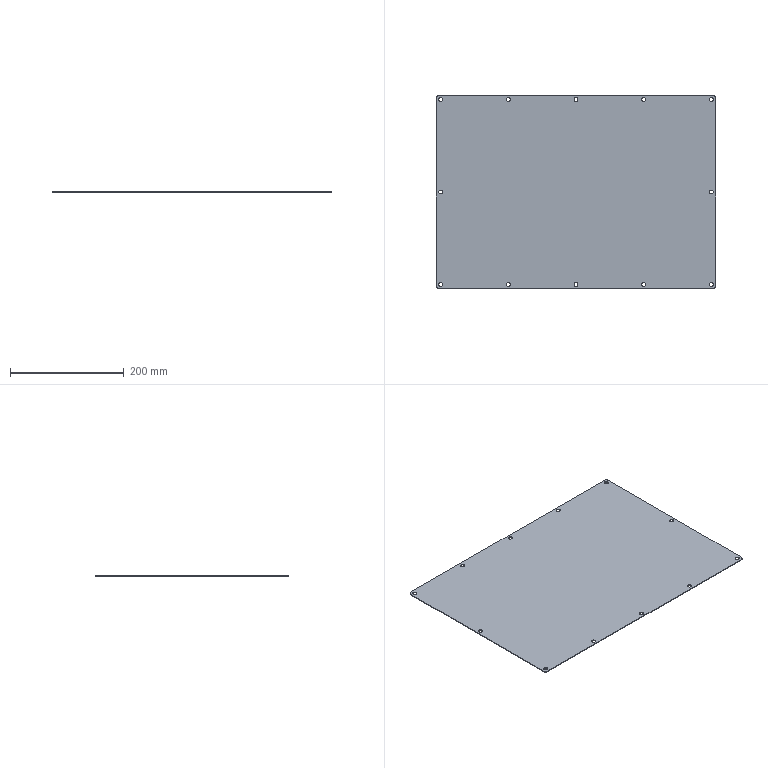Part | SolidWorks | features FlatPattern 1, SMBaseFlange 1, SheetMetal 1 | 1 solid | 34 faces | box 490 x 340 x 1.2 mm | volume 199340 mm3 | cylinder 28 | plane 6 | commonest cylinder face diameters 7 x24 10 x4
STEP:
#1=CARTESIAN_POINT('',(235.2,162.5,1.2));
#2=VERTEX_POINT('',#1);
#3=CARTESIAN_POINT('',(242.2,162.5,1.2));
#4=VERTEX_POINT('',#3);
#5=CARTESIAN_POINT('',(238.7,162.5,1.2));
#6=DIRECTION('',(0.,0.,1.));
#7=DIRECTION('',(1.,0.,0.));
#8=AXIS2_PLACEMENT_3D('',#5,#6,#7);
#9=CIRCLE('',#8,3.5);
#10=EDGE_CURVE('',#2,#4,#9,.T.);
#11=ORIENTED_EDGE('',*,*,#10,.T.);
#12=CARTESIAN_POINT('',(242.2,162.5,0.));
#13=VERTEX_POINT('',#12);
#14=CARTESIAN_POINT('',(242.2,162.5,1.2));
#15=DIRECTION('',(0.,0.,-1.));
#16=VECTOR('',#15,1000.);
#17=LINE('',#14,#16);
#18=EDGE_CURVE('',#4,#13,#17,.T.);
#19=ORIENTED_EDGE('',*,*,#18,.T.);
#20=CARTESIAN_POINT('',(235.2,162.5,0.));
#21=VERTEX_POINT('',#20);
#22=CARTESIAN_POINT('',(238.7,162.5,0.));
#23=DIRECTION('',(0.,0.,1.));
#24=DIRECTION('',(1.,0.,0.));
#25=AXIS2_PLACEMENT_3D('',#22,#23,#24);
#26=CIRCLE('',#25,3.5);
#27=EDGE_CURVE('',#21,#13,#26,.T.);
#28=ORIENTED_EDGE('',*,*,#27,.F.);
#29=CARTESIAN_POINT('',(235.2,162.5,1.2));
#30=DIRECTION('',(0.,0.,-1.));
#31=VECTOR('',#30,1000.);
#32=LINE('',#29,#31);
#33=EDGE_CURVE('',#2,#21,#32,.T.);
#34=ORIENTED_EDGE('',*,*,#33,.F.);
#35=EDGE_LOOP('',(#11,#19,#28,#34));
#36=FACE_OUTER_BOUND('',#35,.T.);
#37=CARTESIAN_POINT('',(238.7,162.5,1.2));
#38=DIRECTION('',(0.,0.,-1.));
#39=DIRECTION('',(-1.,0.,0.));
#40=AXIS2_PLACEMENT_3D('',#37,#38,#39);
#41=CYLINDRICAL_SURFACE('',#40,3.5);
#42=ADVANCED_FACE('',(#36),#41,.F.);
#43=CARTESIAN_POINT('',(235.2,-162.5,1.2));
#44=VERTEX_POINT('',#43);
#45=CARTESIAN_POINT('',(242.2,-162.5,1.2));
#46=VERTEX_POINT('',#45);
#47=CARTESIAN_POINT('',(238.7,-162.5,1.2));
#48=DIRECTION('',(0.,0.,1.));
#49=DIRECTION('',(1.,0.,0.));
#50=AXIS2_PLACEMENT_3D('',#47,#48,#49);
#51=CIRCLE('',#50,3.5);
#52=EDGE_CURVE('',#44,#46,#51,.T.);
#53=ORIENTED_EDGE('',*,*,#52,.T.);
#54=CARTESIAN_POINT('',(242.2,-162.5,0.));
#55=VERTEX_POINT('',#54);
#56=CARTESIAN_POINT('',(242.2,-162.5,1.2));
#57=DIRECTION('',(0.,0.,-1.));
#58=VECTOR('',#57,1000.);
#59=LINE('',#56,#58);
#60=EDGE_CURVE('',#46,#55,#59,.T.);
#61=ORIENTED_EDGE('',*,*,#60,.T.);
#62=CARTESIAN_POINT('',(235.2,-162.5,0.));
#63=VERTEX_POINT('',#62);
#64=CARTESIAN_POINT('',(238.7,-162.5,0.));
#65=DIRECTION('',(0.,0.,1.));
#66=DIRECTION('',(1.,0.,0.));
#67=AXIS2_PLACEMENT_3D('',#64,#65,#66);
#68=CIRCLE('',#67,3.5);
#69=EDGE_CURVE('',#63,#55,#68,.T.);
#70=ORIENTED_EDGE('',*,*,#69,.F.);
#71=CARTESIAN_POINT('',(235.2,-162.5,1.2));
#72=DIRECTION('',(0.,0.,-1.));
#73=VECTOR('',#72,1000.);
#74=LINE('',#71,#73);
#75=EDGE_CURVE('',#44,#63,#74,.T.);
#76=ORIENTED_EDGE('',*,*,#75,.F.);
#77=EDGE_LOOP('',(#53,#61,#70,#76));
#78=FACE_OUTER_BOUND('',#77,.T.);
#79=CARTESIAN_POINT('',(238.7,-162.5,1.2));
#80=DIRECTION('',(0.,0.,-1.));
#81=DIRECTION('',(-1.,0.,0.));
#82=AXIS2_PLACEMENT_3D('',#79,#80,#81);
#83=CYLINDRICAL_SURFACE('',#82,3.5);
#84=ADVANCED_FACE('',(#78),#83,.F.);
#85=CARTESIAN_POINT('',(116.45,162.5,1.2));
#86=VERTEX_POINT('',#85);
#87=CARTESIAN_POINT('',(123.45,162.5,1.2));
#88=VERTEX_POINT('',#87);
#89=CARTESIAN_POINT('',(119.95,162.5,1.2));
#90=DIRECTION('',(0.,0.,1.));
#91=DIRECTION('',(1.,0.,0.));
#92=AXIS2_PLACEMENT_3D('',#89,#90,#91);
#93=CIRCLE('',#92,3.5);
#94=EDGE_CURVE('',#86,#88,#93,.T.);
#95=ORIENTED_EDGE('',*,*,#94,.T.);
#96=CARTESIAN_POINT('',(123.45,162.5,0.));
#97=VERTEX_POINT('',#96);
#98=CARTESIAN_POINT('',(123.45,162.5,1.2));
#99=DIRECTION('',(0.,0.,-1.));
#100=VECTOR('',#99,1000.);
#101=LINE('',#98,#100);
#102=EDGE_CURVE('',#88,#97,#101,.T.);
#103=ORIENTED_EDGE('',*,*,#102,.T.);
#104=CARTESIAN_POINT('',(116.45,162.5,0.));
#105=VERTEX_POINT('',#104);
#106=CARTESIAN_POINT('',(119.95,162.5,0.));
#107=DIRECTION('',(0.,0.,1.));
#108=DIRECTION('',(1.,0.,0.));
#109=AXIS2_PLACEMENT_3D('',#106,#107,#108);
#110=CIRCLE('',#109,3.5);
#111=EDGE_CURVE('',#105,#97,#110,.T.);
#112=ORIENTED_EDGE('',*,*,#111,.F.);
#113=CARTESIAN_POINT('',(116.45,162.5,1.2));
#114=DIRECTION('',(0.,0.,-1.));
#115=VECTOR('',#114,1000.);
#116=LINE('',#113,#115);
#117=EDGE_CURVE('',#86,#105,#116,.T.);
#118=ORIENTED_EDGE('',*,*,#117,.F.);
#119=EDGE_LOOP('',(#95,#103,#112,#118));
#120=FACE_OUTER_BOUND('',#119,.T.);
#121=CARTESIAN_POINT('',(119.95,162.5,1.2));
#122=DIRECTION('',(0.,0.,-1.));
#123=DIRECTION('',(-1.,0.,0.));
#124=AXIS2_PLACEMENT_3D('',#121,#122,#123);
#125=CYLINDRICAL_SURFACE('',#124,3.5);
#126=ADVANCED_FACE('',(#120),#125,.F.);
#127=CARTESIAN_POINT('',(116.45,-162.5,1.2));
#128=VERTEX_POINT('',#127);
#129=CARTESIAN_POINT('',(123.45,-162.5,1.2));
#130=VERTEX_POINT('',#129);
#131=CARTESIAN_POINT('',(119.95,-162.5,1.2));
#132=DIRECTION('',(0.,0.,1.));
#133=DIRECTION('',(1.,0.,0.));
#134=AXIS2_PLACEMENT_3D('',#131,#132,#133);
#135=CIRCLE('',#134,3.5);
#136=EDGE_CURVE('',#128,#130,#135,.T.);
#137=ORIENTED_EDGE('',*,*,#136,.T.);
#138=CARTESIAN_POINT('',(123.45,-162.5,0.));
#139=VERTEX_POINT('',#138);
#140=CARTESIAN_POINT('',(123.45,-162.5,1.2));
#141=DIRECTION('',(0.,0.,-1.));
#142=VECTOR('',#141,1000.);
#143=LINE('',#140,#142);
#144=EDGE_CURVE('',#130,#139,#143,.T.);
#145=ORIENTED_EDGE('',*,*,#144,.T.);
#146=CARTESIAN_POINT('',(116.45,-162.5,0.));
#147=VERTEX_POINT('',#146);
#148=CARTESIAN_POINT('',(119.95,-162.5,0.));
#149=DIRECTION('',(0.,0.,1.));
#150=DIRECTION('',(1.,0.,0.));
#151=AXIS2_PLACEMENT_3D('',#148,#149,#150);
#152=CIRCLE('',#151,3.5);
#153=EDGE_CURVE('',#147,#139,#152,.T.);
#154=ORIENTED_EDGE('',*,*,#153,.F.);
#155=CARTESIAN_POINT('',(116.45,-162.5,1.2));
#156=DIRECTION('',(0.,0.,-1.));
#157=VECTOR('',#156,1000.);
#158=LINE('',#155,#157);
#159=EDGE_CURVE('',#128,#147,#158,.T.);
#160=ORIENTED_EDGE('',*,*,#159,.F.);
#161=EDGE_LOOP('',(#137,#145,#154,#160));
#162=FACE_OUTER_BOUND('',#161,.T.);
#163=CARTESIAN_POINT('',(119.95,-162.5,1.2));
#164=DIRECTION('',(0.,0.,-1.));
#165=DIRECTION('',(-1.,0.,0.));
#166=AXIS2_PLACEMENT_3D('',#163,#164,#165);
#167=CYLINDRICAL_SURFACE('',#166,3.5);
#168=ADVANCED_FACE('',(#162),#167,.F.);
#169=CARTESIAN_POINT('',(-2.3,162.5,1.2));
#170=VERTEX_POINT('',#169);
#171=CARTESIAN_POINT('',(4.7,162.5,1.2));
#172=VERTEX_POINT('',#171);
#173=CARTESIAN_POINT('',(1.2,162.5,1.2));
#174=DIRECTION('',(0.,0.,1.));
#175=DIRECTION('',(1.,0.,0.));
#176=AXIS2_PLACEMENT_3D('',#173,#174,#175);
#177=CIRCLE('',#176,3.5);
#178=EDGE_CURVE('',#170,#172,#177,.T.);
#179=ORIENTED_EDGE('',*,*,#178,.T.);
#180=CARTESIAN_POINT('',(4.7,162.5,0.));
#181=VERTEX_POINT('',#180);
#182=CARTESIAN_POINT('',(4.7,162.5,1.2));
#183=DIRECTION('',(0.,0.,-1.));
#184=VECTOR('',#183,1000.);
#185=LINE('',#182,#184);
#186=EDGE_CURVE('',#172,#181,#185,.T.);
#187=ORIENTED_EDGE('',*,*,#186,.T.);
#188=CARTESIAN_POINT('',(-2.3,162.5,0.));
#189=VERTEX_POINT('',#188);
#190=CARTESIAN_POINT('',(1.2,162.5,0.));
#191=DIRECTION('',(0.,0.,1.));
#192=DIRECTION('',(1.,0.,0.));
#193=AXIS2_PLACEMENT_3D('',#190,#191,#192);
#194=CIRCLE('',#193,3.5);
#195=EDGE_CURVE('',#189,#181,#194,.T.);
#196=ORIENTED_EDGE('',*,*,#195,.F.);
#197=CARTESIAN_POINT('',(-2.3,162.5,1.2));
#198=DIRECTION('',(0.,0.,-1.));
#199=VECTOR('',#198,1000.);
#200=LINE('',#197,#199);
#201=EDGE_CURVE('',#170,#189,#200,.T.);
#202=ORIENTED_EDGE('',*,*,#201,.F.);
#203=EDGE_LOOP('',(#179,#187,#196,#202));
#204=FACE_OUTER_BOUND('',#203,.T.);
#205=CARTESIAN_POINT('',(1.2,162.5,1.2));
#206=DIRECTION('',(0.,0.,-1.));
#207=DIRECTION('',(-1.,0.,0.));
#208=AXIS2_PLACEMENT_3D('',#205,#206,#207);
#209=CYLINDRICAL_SURFACE('',#208,3.5);
#210=ADVANCED_FACE('',(#204),#209,.F.);
#211=CARTESIAN_POINT('',(-2.3,-162.5,1.2));
#212=VERTEX_POINT('',#211);
#213=CARTESIAN_POINT('',(4.7,-162.5,1.2));
#214=VERTEX_POINT('',#213);
#215=CARTESIAN_POINT('',(1.2,-162.5,1.2));
#216=DIRECTION('',(0.,0.,1.));
#217=DIRECTION('',(1.,0.,0.));
#218=AXIS2_PLACEMENT_3D('',#215,#216,#217);
#219=CIRCLE('',#218,3.5);
#220=EDGE_CURVE('',#212,#214,#219,.T.);
#221=ORIENTED_EDGE('',*,*,#220,.T.);
#222=CARTESIAN_POINT('',(4.7,-162.5,0.));
#223=VERTEX_POINT('',#222);
#224=CARTESIAN_POINT('',(4.7,-162.5,1.2));
#225=DIRECTION('',(0.,0.,-1.));
#226=VECTOR('',#225,1000.);
#227=LINE('',#224,#226);
#228=EDGE_CURVE('',#214,#223,#227,.T.);
#229=ORIENTED_EDGE('',*,*,#228,.T.);
#230=CARTESIAN_POINT('',(-2.3,-162.5,0.));
#231=VERTEX_POINT('',#230);
#232=CARTESIAN_POINT('',(1.2,-162.5,0.));
#233=DIRECTION('',(0.,0.,1.));
#234=DIRECTION('',(1.,0.,0.));
#235=AXIS2_PLACEMENT_3D('',#232,#233,#234);
#236=CIRCLE('',#235,3.5);
#237=EDGE_CURVE('',#231,#223,#236,.T.);
#238=ORIENTED_EDGE('',*,*,#237,.F.);
#239=CARTESIAN_POINT('',(-2.3,-162.5,1.2));
#240=DIRECTION('',(0.,0.,-1.));
#241=VECTOR('',#240,1000.);
#242=LINE('',#239,#241);
#243=EDGE_CURVE('',#212,#231,#242,.T.);
#244=ORIENTED_EDGE('',*,*,#243,.F.);
#245=EDGE_LOOP('',(#221,#229,#238,#244));
#246=FACE_OUTER_BOUND('',#245,.T.);
#247=CARTESIAN_POINT('',(1.2,-162.5,1.2));
#248=DIRECTION('',(0.,0.,-1.));
#249=DIRECTION('',(-1.,0.,0.));
#250=AXIS2_PLACEMENT_3D('',#247,#248,#249);
#251=CYLINDRICAL_SURFACE('',#250,3.5);
#252=ADVANCED_FACE('',(#246),#251,.F.);
#253=CARTESIAN_POINT('',(-121.05,162.5,1.2));
#254=VERTEX_POINT('',#253);
#255=CARTESIAN_POINT('',(-114.05,162.5,1.2));
#256=VERTEX_POINT('',#255);
#257=CARTESIAN_POINT('',(-117.55,162.5,1.2));
#258=DIRECTION('',(0.,0.,1.));
#259=DIRECTION('',(1.,0.,0.));
#260=AXIS2_PLACEMENT_3D('',#257,#258,#259);
#261=CIRCLE('',#260,3.5);
#262=EDGE_CURVE('',#254,#256,#261,.T.);
#263=ORIENTED_EDGE('',*,*,#262,.T.);
#264=CARTESIAN_POINT('',(-114.05,162.5,0.));
#265=VERTEX_POINT('',#264);
#266=CARTESIAN_POINT('',(-114.05,162.5,1.2));
#267=DIRECTION('',(0.,0.,-1.));
#268=VECTOR('',#267,1000.);
#269=LINE('',#266,#268);
#270=EDGE_CURVE('',#256,#265,#269,.T.);
#271=ORIENTED_EDGE('',*,*,#270,.T.);
#272=CARTESIAN_POINT('',(-121.05,162.5,0.));
#273=VERTEX_POINT('',#272);
#274=CARTESIAN_POINT('',(-117.55,162.5,0.));
#275=DIRECTION('',(0.,0.,1.));
#276=DIRECTION('',(1.,0.,0.));
#277=AXIS2_PLACEMENT_3D('',#274,#275,#276);
#278=CIRCLE('',#277,3.5);
#279=EDGE_CURVE('',#273,#265,#278,.T.);
#280=ORIENTED_EDGE('',*,*,#279,.F.);
#281=CARTESIAN_POINT('',(-121.05,162.5,1.2));
#282=DIRECTION('',(0.,0.,-1.));
#283=VECTOR('',#282,1000.);
#284=LINE('',#281,#283);
#285=EDGE_CURVE('',#254,#273,#284,.T.);
#286=ORIENTED_EDGE('',*,*,#285,.F.);
#287=EDGE_LOOP('',(#263,#271,#280,#286));
#288=FACE_OUTER_BOUND('',#287,.T.);
#289=CARTESIAN_POINT('',(-117.55,162.5,1.2));
#290=DIRECTION('',(0.,0.,-1.));
#291=DIRECTION('',(-1.,0.,0.));
#292=AXIS2_PLACEMENT_3D('',#289,#290,#291);
#293=CYLINDRICAL_SURFACE('',#292,3.5);
#294=ADVANCED_FACE('',(#288),#293,.F.);
#295=CARTESIAN_POINT('',(-121.05,-162.5,1.2));
#296=VERTEX_POINT('',#295);
#297=CARTESIAN_POINT('',(-114.05,-162.5,1.2));
#298=VERTEX_POINT('',#297);
#299=CARTESIAN_POINT('',(-117.55,-162.5,1.2));
#300=DIRECTION('',(0.,0.,1.));
#301=DIRECTION('',(1.,0.,0.));
#302=AXIS2_PLACEMENT_3D('',#299,#300,#301);
#303=CIRCLE('',#302,3.5);
#304=EDGE_CURVE('',#296,#298,#303,.T.);
#305=ORIENTED_EDGE('',*,*,#304,.T.);
#306=CARTESIAN_POINT('',(-114.05,-162.5,0.));
#307=VERTEX_POINT('',#306);
#308=CARTESIAN_POINT('',(-114.05,-162.5,1.2));
#309=DIRECTION('',(0.,0.,-1.));
#310=VECTOR('',#309,1000.);
#311=LINE('',#308,#310);
#312=EDGE_CURVE('',#298,#307,#311,.T.);
#313=ORIENTED_EDGE('',*,*,#312,.T.);
#314=CARTESIAN_POINT('',(-121.05,-162.5,0.));
#315=VERTEX_POINT('',#314);
#316=CARTESIAN_POINT('',(-117.55,-162.5,0.));
#317=DIRECTION('',(0.,0.,1.));
#318=DIRECTION('',(1.,0.,0.));
#319=AXIS2_PLACEMENT_3D('',#316,#317,#318);
#320=CIRCLE('',#319,3.5);
#321=EDGE_CURVE('',#315,#307,#320,.T.);
#322=ORIENTED_EDGE('',*,*,#321,.F.);
#323=CARTESIAN_POINT('',(-121.05,-162.5,1.2));
#324=DIRECTION('',(0.,0.,-1.));
#325=VECTOR('',#324,1000.);
#326=LINE('',#323,#325);
#327=EDGE_CURVE('',#296,#315,#326,.T.);
#328=ORIENTED_EDGE('',*,*,#327,.F.);
#329=EDGE_LOOP('',(#305,#313,#322,#328));
#330=FACE_OUTER_BOUND('',#329,.T.);
#331=CARTESIAN_POINT('',(-117.55,-162.5,1.2));
#332=DIRECTION('',(0.,0.,-1.));
#333=DIRECTION('',(-1.,0.,0.));
#334=AXIS2_PLACEMENT_3D('',#331,#332,#333);
#335=CYLINDRICAL_SURFACE('',#334,3.5);
#336=ADVANCED_FACE('',(#330),#335,.F.);
#337=CARTESIAN_POINT('',(235.2,0.,1.2));
#338=VERTEX_POINT('',#337);
#339=CARTESIAN_POINT('',(242.2,0.,1.2));
#340=VERTEX_POINT('',#339);
#341=CARTESIAN_POINT('',(238.7,0.,1.2));
#342=DIRECTION('',(0.,0.,1.));
#343=DIRECTION('',(1.,0.,0.));
#344=AXIS2_PLACEMENT_3D('',#341,#342,#343);
#345=CIRCLE('',#344,3.5);
#346=EDGE_CURVE('',#338,#340,#345,.T.);
#347=ORIENTED_EDGE('',*,*,#346,.T.);
#348=CARTESIAN_POINT('',(242.2,0.,0.));
#349=VERTEX_POINT('',#348);
#350=CARTESIAN_POINT('',(242.2,0.,1.2));
#351=DIRECTION('',(0.,0.,-1.));
#352=VECTOR('',#351,1000.);
#353=LINE('',#350,#352);
#354=EDGE_CURVE('',#340,#349,#353,.T.);
#355=ORIENTED_EDGE('',*,*,#354,.T.);
#356=CARTESIAN_POINT('',(235.2,0.,0.));
#357=VERTEX_POINT('',#356);
#358=CARTESIAN_POINT('',(238.7,0.,0.));
#359=DIRECTION('',(0.,0.,1.));
#360=DIRECTION('',(1.,0.,0.));
#361=AXIS2_PLACEMENT_3D('',#358,#359,#360);
#362=CIRCLE('',#361,3.5);
#363=EDGE_CURVE('',#357,#349,#362,.T.);
#364=ORIENTED_EDGE('',*,*,#363,.F.);
#365=CARTESIAN_POINT('',(235.2,0.,1.2));
#366=DIRECTION('',(0.,0.,-1.));
#367=VECTOR('',#366,1000.);
#368=LINE('',#365,#367);
#369=EDGE_CURVE('',#338,#357,#368,.T.);
#370=ORIENTED_EDGE('',*,*,#369,.F.);
#371=EDGE_LOOP('',(#347,#355,#364,#370));
#372=FACE_OUTER_BOUND('',#371,.T.);
#373=CARTESIAN_POINT('',(238.7,0.,1.2));
#374=DIRECTION('',(0.,0.,-1.));
#375=DIRECTION('',(-1.,0.,0.));
#376=AXIS2_PLACEMENT_3D('',#373,#374,#375);
#377=CYLINDRICAL_SURFACE('',#376,3.5);
#378=ADVANCED_FACE('',(#372),#377,.F.);
#379=CARTESIAN_POINT('',(-239.8,162.5,1.2));
#380=VERTEX_POINT('',#379);
#381=CARTESIAN_POINT('',(-232.8,162.5,1.2));
#382=VERTEX_POINT('',#381);
#383=CARTESIAN_POINT('',(-236.3,162.5,1.2));
#384=DIRECTION('',(0.,0.,1.));
#385=DIRECTION('',(1.,0.,0.));
#386=AXIS2_PLACEMENT_3D('',#383,#384,#385);
#387=CIRCLE('',#386,3.5);
#388=EDGE_CURVE('',#380,#382,#387,.T.);
#389=ORIENTED_EDGE('',*,*,#388,.T.);
#390=CARTESIAN_POINT('',(-232.8,162.5,0.));
#391=VERTEX_POINT('',#390);
#392=CARTESIAN_POINT('',(-232.8,162.5,1.2));
#393=DIRECTION('',(0.,0.,-1.));
#394=VECTOR('',#393,1000.);
#395=LINE('',#392,#394);
#396=EDGE_CURVE('',#382,#391,#395,.T.);
#397=ORIENTED_EDGE('',*,*,#396,.T.);
#398=CARTESIAN_POINT('',(-239.8,162.5,0.));
#399=VERTEX_POINT('',#398);
#400=CARTESIAN_POINT('',(-236.3,162.5,0.));
#401=DIRECTION('',(0.,0.,1.));
#402=DIRECTION('',(1.,0.,0.));
#403=AXIS2_PLACEMENT_3D('',#400,#401,#402);
#404=CIRCLE('',#403,3.5);
#405=EDGE_CURVE('',#399,#391,#404,.T.);
#406=ORIENTED_EDGE('',*,*,#405,.F.);
#407=CARTESIAN_POINT('',(-239.8,162.5,1.2));
#408=DIRECTION('',(0.,0.,-1.));
#409=VECTOR('',#408,1000.);
#410=LINE('',#407,#409);
#411=EDGE_CURVE('',#380,#399,#410,.T.);
#412=ORIENTED_EDGE('',*,*,#411,.F.);
#413=EDGE_LOOP('',(#389,#397,#406,#412));
#414=FACE_OUTER_BOUND('',#413,.T.);
#415=CARTESIAN_POINT('',(-236.3,162.5,1.2));
#416=DIRECTION('',(0.,0.,-1.));
#417=DIRECTION('',(-1.,0.,0.));
#418=AXIS2_PLACEMENT_3D('',#415,#416,#417);
#419=CYLINDRICAL_SURFACE('',#418,3.5);
#420=ADVANCED_FACE('',(#414),#419,.F.);
#421=CARTESIAN_POINT('',(-239.8,0.,1.2));
#422=VERTEX_POINT('',#421);
#423=CARTESIAN_POINT('',(-232.8,0.,1.2));
#424=VERTEX_POINT('',#423);
#425=CARTESIAN_POINT('',(-236.3,0.,1.2));
#426=DIRECTION('',(0.,0.,1.));
#427=DIRECTION('',(1.,0.,0.));
#428=AXIS2_PLACEMENT_3D('',#425,#426,#427);
#429=CIRCLE('',#428,3.5);
#430=EDGE_CURVE('',#422,#424,#429,.T.);
#431=ORIENTED_EDGE('',*,*,#430,.T.);
#432=CARTESIAN_POINT('',(-232.8,0.,0.));
#433=VERTEX_POINT('',#432);
#434=CARTESIAN_POINT('',(-232.8,0.,1.2));
#435=DIRECTION('',(0.,0.,-1.));
#436=VECTOR('',#435,1000.);
#437=LINE('',#434,#436);
#438=EDGE_CURVE('',#424,#433,#437,.T.);
#439=ORIENTED_EDGE('',*,*,#438,.T.);
#440=CARTESIAN_POINT('',(-239.8,0.,0.));
#441=VERTEX_POINT('',#440);
#442=CARTESIAN_POINT('',(-236.3,0.,0.));
#443=DIRECTION('',(0.,0.,1.));
#444=DIRECTION('',(1.,0.,0.));
#445=AXIS2_PLACEMENT_3D('',#442,#443,#444);
#446=CIRCLE('',#445,3.5);
#447=EDGE_CURVE('',#441,#433,#446,.T.);
#448=ORIENTED_EDGE('',*,*,#447,.F.);
#449=CARTESIAN_POINT('',(-239.8,0.,1.2));
#450=DIRECTION('',(0.,0.,-1.));
#451=VECTOR('',#450,1000.);
#452=LINE('',#449,#451);
#453=EDGE_CURVE('',#422,#441,#452,.T.);
#454=ORIENTED_EDGE('',*,*,#453,.F.);
#455=EDGE_LOOP('',(#431,#439,#448,#454));
#456=FACE_OUTER_BOUND('',#455,.T.);
#457=CARTESIAN_POINT('',(-236.3,0.,1.2));
#458=DIRECTION('',(0.,0.,-1.));
#459=DIRECTION('',(-1.,0.,0.));
#460=AXIS2_PLACEMENT_3D('',#457,#458,#459);
#461=CYLINDRICAL_SURFACE('',#460,3.5);
#462=ADVANCED_FACE('',(#456),#461,.F.);
#463=CARTESIAN_POINT('',(-239.8,-162.5,1.2));
#464=VERTEX_POINT('',#463);
#465=CARTESIAN_POINT('',(-232.8,-162.5,1.2));
#466=VERTEX_POINT('',#465);
#467=CARTESIAN_POINT('',(-236.3,-162.5,1.2));
#468=DIRECTION('',(0.,0.,1.));
#469=DIRECTION('',(1.,0.,0.));
#470=AXIS2_PLACEMENT_3D('',#467,#468,#469);
#471=CIRCLE('',#470,3.5);
#472=EDGE_CURVE('',#464,#466,#471,.T.);
#473=ORIENTED_EDGE('',*,*,#472,.T.);
#474=CARTESIAN_POINT('',(-232.8,-162.5,0.));
#475=VERTEX_POINT('',#474);
#476=CARTESIAN_POINT('',(-232.8,-162.5,1.2));
#477=DIRECTION('',(0.,0.,-1.));
#478=VECTOR('',#477,1000.);
#479=LINE('',#476,#478);
#480=EDGE_CURVE('',#466,#475,#479,.T.);
#481=ORIENTED_EDGE('',*,*,#480,.T.);
#482=CARTESIAN_POINT('',(-239.8,-162.5,0.));
#483=VERTEX_POINT('',#482);
#484=CARTESIAN_POINT('',(-236.3,-162.5,0.));
#485=DIRECTION('',(0.,0.,1.));
#486=DIRECTION('',(1.,0.,0.));
#487=AXIS2_PLACEMENT_3D('',#484,#485,#486);
#488=CIRCLE('',#487,3.5);
#489=EDGE_CURVE('',#483,#475,#488,.T.);
#490=ORIENTED_EDGE('',*,*,#489,.F.);
#491=CARTESIAN_POINT('',(-239.8,-162.5,1.2));
#492=DIRECTION('',(0.,0.,-1.));
#493=VECTOR('',#492,1000.);
#494=LINE('',#491,#493);
#495=EDGE_CURVE('',#464,#483,#494,.T.);
#496=ORIENTED_EDGE('',*,*,#495,.F.);
#497=EDGE_LOOP('',(#473,#481,#490,#496));
#498=FACE_OUTER_BOUND('',#497,.T.);
#499=CARTESIAN_POINT('',(-236.3,-162.5,1.2));
#500=DIRECTION('',(0.,0.,-1.));
#501=DIRECTION('',(-1.,0.,0.));
#502=AXIS2_PLACEMENT_3D('',#499,#500,#501);
#503=CYLINDRICAL_SURFACE('',#502,3.5);
#504=ADVANCED_FACE('',(#498),#503,.F.);
#505=ORIENTED_EDGE('',*,*,#52,.F.);
#506=CARTESIAN_POINT('',(238.7,-162.5,1.2));
#507=DIRECTION('',(0.,0.,1.));
#508=DIRECTION('',(1.,0.,0.));
#509=AXIS2_PLACEMENT_3D('',#506,#507,#508);
#510=CIRCLE('',#509,3.5);
#511=EDGE_CURVE('',#46,#44,#510,.T.);
#512=ORIENTED_EDGE('',*,*,#511,.F.);
#513=EDGE_LOOP('',(#505,#512));
#514=FACE_BOUND('',#513,.T.);
#515=ORIENTED_EDGE('',*,*,#136,.F.);
#516=CARTESIAN_POINT('',(119.95,-162.5,1.2));
#517=DIRECTION('',(0.,0.,1.));
#518=DIRECTION('',(1.,0.,0.));
#519=AXIS2_PLACEMENT_3D('',#516,#517,#518);
#520=CIRCLE('',#519,3.5);
#521=EDGE_CURVE('',#130,#128,#520,.T.);
#522=ORIENTED_EDGE('',*,*,#521,.F.);
#523=EDGE_LOOP('',(#515,#522));
#524=FACE_BOUND('',#523,.T.);
#525=ORIENTED_EDGE('',*,*,#220,.F.);
#526=CARTESIAN_POINT('',(1.2,-162.5,1.2));
#527=DIRECTION('',(0.,0.,1.));
#528=DIRECTION('',(1.,0.,0.));
#529=AXIS2_PLACEMENT_3D('',#526,#527,#528);
#530=CIRCLE('',#529,3.5);
#531=EDGE_CURVE('',#214,#212,#530,.T.);
#532=ORIENTED_EDGE('',*,*,#531,.F.);
#533=EDGE_LOOP('',(#525,#532));
#534=FACE_BOUND('',#533,.T.);
#535=ORIENTED_EDGE('',*,*,#304,.F.);
#536=CARTESIAN_POINT('',(-117.55,-162.5,1.2));
#537=DIRECTION('',(0.,0.,1.));
#538=DIRECTION('',(1.,0.,0.));
#539=AXIS2_PLACEMENT_3D('',#536,#537,#538);
#540=CIRCLE('',#539,3.5);
#541=EDGE_CURVE('',#298,#296,#540,.T.);
#542=ORIENTED_EDGE('',*,*,#541,.F.);
#543=EDGE_LOOP('',(#535,#542));
#544=FACE_BOUND('',#543,.T.);
#545=ORIENTED_EDGE('',*,*,#388,.F.);
#546=CARTESIAN_POINT('',(-236.3,162.5,1.2));
#547=DIRECTION('',(0.,0.,1.));
#548=DIRECTION('',(1.,0.,0.));
#549=AXIS2_PLACEMENT_3D('',#546,#547,#548);
#550=CIRCLE('',#549,3.5);
#551=EDGE_CURVE('',#382,#380,#550,.T.);
#552=ORIENTED_EDGE('',*,*,#551,.F.);
#553=EDGE_LOOP('',(#545,#552));
#554=FACE_BOUND('',#553,.T.);
#555=ORIENTED_EDGE('',*,*,#472,.F.);
#556=CARTESIAN_POINT('',(-236.3,-162.5,1.2));
#557=DIRECTION('',(0.,0.,1.));
#558=DIRECTION('',(1.,0.,0.));
#559=AXIS2_PLACEMENT_3D('',#556,#557,#558);
#560=CIRCLE('',#559,3.5);
#561=EDGE_CURVE('',#466,#464,#560,.T.);
#562=ORIENTED_EDGE('',*,*,#561,.F.);
#563=EDGE_LOOP('',(#555,#562));
#564=FACE_BOUND('',#563,.T.);
#565=CARTESIAN_POINT('',(241.2,-170.,1.2));
#566=VERTEX_POINT('',#565);
#567=CARTESIAN_POINT('',(246.2,-165.,1.2));
#568=VERTEX_POINT('',#567);
#569=CARTESIAN_POINT('',(241.2,-165.,1.2));
#570=DIRECTION('',(0.,0.,1.));
#571=DIRECTION('',(1.,0.,0.));
#572=AXIS2_PLACEMENT_3D('',#569,#570,#571);
#573=CIRCLE('',#572,5.);
#574=EDGE_CURVE('',#566,#568,#573,.T.);
#575=ORIENTED_EDGE('',*,*,#574,.T.);
#576=CARTESIAN_POINT('',(246.2,165.,1.2));
#577=VERTEX_POINT('',#576);
#578=CARTESIAN_POINT('',(246.2,-165.,1.2));
#579=DIRECTION('',(0.,1.,0.));
#580=VECTOR('',#579,1000.);
#581=LINE('',#578,#580);
#582=EDGE_CURVE('',#568,#577,#581,.T.);
#583=ORIENTED_EDGE('',*,*,#582,.T.);
#584=CARTESIAN_POINT('',(241.2,170.,1.2));
#585=VERTEX_POINT('',#584);
#586=CARTESIAN_POINT('',(241.2,165.,1.2));
#587=DIRECTION('',(0.,0.,1.));
#588=DIRECTION('',(-1.,0.,0.));
#589=AXIS2_PLACEMENT_3D('',#586,#587,#588);
#590=CIRCLE('',#589,5.);
#591=EDGE_CURVE('',#577,#585,#590,.T.);
#592=ORIENTED_EDGE('',*,*,#591,.T.);
#593=CARTESIAN_POINT('',(-238.8,170.,1.2));
#594=VERTEX_POINT('',#593);
#595=CARTESIAN_POINT('',(-238.8,170.,1.2));
#596=DIRECTION('',(-1.,0.,0.));
#597=VECTOR('',#596,1000.);
#598=LINE('',#595,#597);
#599=EDGE_CURVE('',#585,#594,#598,.T.);
#600=ORIENTED_EDGE('',*,*,#599,.T.);
#601=CARTESIAN_POINT('',(-243.8,165.,1.2));
#602=VERTEX_POINT('',#601);
#603=CARTESIAN_POINT('',(-238.8,165.,1.2));
#604=DIRECTION('',(0.,0.,1.));
#605=DIRECTION('',(-1.,0.,0.));
#606=AXIS2_PLACEMENT_3D('',#603,#604,#605);
#607=CIRCLE('',#606,5.);
#608=EDGE_CURVE('',#594,#602,#607,.T.);
#609=ORIENTED_EDGE('',*,*,#608,.T.);
#610=CARTESIAN_POINT('',(-243.8,-165.,1.2));
#611=VERTEX_POINT('',#610);
#612=CARTESIAN_POINT('',(-243.8,-165.,1.2));
#613=DIRECTION('',(0.,-1.,0.));
#614=VECTOR('',#613,1000.);
#615=LINE('',#612,#614);
#616=EDGE_CURVE('',#602,#611,#615,.T.);
#617=ORIENTED_EDGE('',*,*,#616,.T.);
#618=CARTESIAN_POINT('',(-238.8,-170.,1.2));
#619=VERTEX_POINT('',#618);
#620=CARTESIAN_POINT('',(-238.8,-165.,1.2));
#621=DIRECTION('',(0.,0.,1.));
#622=DIRECTION('',(-1.,0.,0.));
#623=AXIS2_PLACEMENT_3D('',#620,#621,#622);
#624=CIRCLE('',#623,5.);
#625=EDGE_CURVE('',#611,#619,#624,.T.);
#626=ORIENTED_EDGE('',*,*,#625,.T.);
#627=CARTESIAN_POINT('',(-238.8,-170.,1.2));
#628=DIRECTION('',(1.,0.,0.));
#629=VECTOR('',#628,1000.);
#630=LINE('',#627,#629);
#631=EDGE_CURVE('',#619,#566,#630,.T.);
#632=ORIENTED_EDGE('',*,*,#631,.T.);
#633=EDGE_LOOP('',(#575,#583,#592,#600,#609,#617,#626,#632));
#634=FACE_OUTER_BOUND('',#633,.T.);
#635=ORIENTED_EDGE('',*,*,#430,.F.);
#636=CARTESIAN_POINT('',(-236.3,0.,1.2));
#637=DIRECTION('',(0.,0.,1.));
#638=DIRECTION('',(1.,0.,0.));
#639=AXIS2_PLACEMENT_3D('',#636,#637,#638);
#640=CIRCLE('',#639,3.5);
#641=EDGE_CURVE('',#424,#422,#640,.T.);
#642=ORIENTED_EDGE('',*,*,#641,.F.);
#643=EDGE_LOOP('',(#635,#642));
#644=FACE_BOUND('',#643,.T.);
#645=ORIENTED_EDGE('',*,*,#346,.F.);
#646=CARTESIAN_POINT('',(238.7,0.,1.2));
#647=DIRECTION('',(0.,0.,1.));
#648=DIRECTION('',(1.,0.,0.));
#649=AXIS2_PLACEMENT_3D('',#646,#647,#648);
#650=CIRCLE('',#649,3.5);
#651=EDGE_CURVE('',#340,#338,#650,.T.);
#652=ORIENTED_EDGE('',*,*,#651,.F.);
#653=EDGE_LOOP('',(#645,#652));
#654=FACE_BOUND('',#653,.T.);
#655=ORIENTED_EDGE('',*,*,#262,.F.);
#656=CARTESIAN_POINT('',(-117.55,162.5,1.2));
#657=DIRECTION('',(0.,0.,1.));
#658=DIRECTION('',(1.,0.,0.));
#659=AXIS2_PLACEMENT_3D('',#656,#657,#658);
#660=CIRCLE('',#659,3.5);
#661=EDGE_CURVE('',#256,#254,#660,.T.);
#662=ORIENTED_EDGE('',*,*,#661,.F.);
#663=EDGE_LOOP('',(#655,#662));
#664=FACE_BOUND('',#663,.T.);
#665=ORIENTED_EDGE('',*,*,#178,.F.);
#666=CARTESIAN_POINT('',(1.2,162.5,1.2));
#667=DIRECTION('',(0.,0.,1.));
#668=DIRECTION('',(1.,0.,0.));
#669=AXIS2_PLACEMENT_3D('',#666,#667,#668);
#670=CIRCLE('',#669,3.5);
#671=EDGE_CURVE('',#172,#170,#670,.T.);
#672=ORIENTED_EDGE('',*,*,#671,.F.);
#673=EDGE_LOOP('',(#665,#672));
#674=FACE_BOUND('',#673,.T.);
#675=ORIENTED_EDGE('',*,*,#94,.F.);
#676=CARTESIAN_POINT('',(119.95,162.5,1.2));
#677=DIRECTION('',(0.,0.,1.));
#678=DIRECTION('',(1.,0.,0.));
#679=AXIS2_PLACEMENT_3D('',#676,#677,#678);
#680=CIRCLE('',#679,3.5);
#681=EDGE_CURVE('',#88,#86,#680,.T.);
#682=ORIENTED_EDGE('',*,*,#681,.F.);
#683=EDGE_LOOP('',(#675,#682));
#684=FACE_BOUND('',#683,.T.);
#685=ORIENTED_EDGE('',*,*,#10,.F.);
#686=CARTESIAN_POINT('',(238.7,162.5,1.2));
#687=DIRECTION('',(0.,0.,1.));
#688=DIRECTION('',(1.,0.,0.));
#689=AXIS2_PLACEMENT_3D('',#686,#687,#688);
#690=CIRCLE('',#689,3.5);
#691=EDGE_CURVE('',#4,#2,#690,.T.);
#692=ORIENTED_EDGE('',*,*,#691,.F.);
#693=EDGE_LOOP('',(#685,#692));
#694=FACE_BOUND('',#693,.T.);
#695=CARTESIAN_POINT('',(241.2,-165.,1.2));
#696=DIRECTION('',(0.,0.,1.));
#697=DIRECTION('',(1.,0.,0.));
#698=AXIS2_PLACEMENT_3D('',#695,#696,#697);
#699=PLANE('',#698);
#700=ADVANCED_FACE('',(#514,#524,#534,#544,#554,#564,#634,#644,#654,#664,#674,#684,#694),#699,.T.);
#701=CARTESIAN_POINT('',(241.2,-170.,0.));
#702=VERTEX_POINT('',#701);
#703=CARTESIAN_POINT('',(246.2,-165.,0.));
#704=VERTEX_POINT('',#703);
#705=CARTESIAN_POINT('',(241.2,-165.,0.));
#706=DIRECTION('',(0.,0.,1.));
#707=DIRECTION('',(1.,0.,0.));
#708=AXIS2_PLACEMENT_3D('',#705,#706,#707);
#709=CIRCLE('',#708,5.);
#710=EDGE_CURVE('',#702,#704,#709,.T.);
#711=ORIENTED_EDGE('',*,*,#710,.F.);
#712=CARTESIAN_POINT('',(-238.8,-170.,0.));
#713=VERTEX_POINT('',#712);
#714=CARTESIAN_POINT('',(-238.8,-170.,0.));
#715=DIRECTION('',(1.,0.,0.));
#716=VECTOR('',#715,1000.);
#717=LINE('',#714,#716);
#718=EDGE_CURVE('',#713,#702,#717,.T.);
#719=ORIENTED_EDGE('',*,*,#718,.F.);
#720=CARTESIAN_POINT('',(-243.8,-165.,0.));
#721=VERTEX_POINT('',#720);
#722=CARTESIAN_POINT('',(-238.8,-165.,0.));
#723=DIRECTION('',(0.,0.,1.));
#724=DIRECTION('',(-1.,0.,0.));
#725=AXIS2_PLACEMENT_3D('',#722,#723,#724);
#726=CIRCLE('',#725,5.);
#727=EDGE_CURVE('',#721,#713,#726,.T.);
#728=ORIENTED_EDGE('',*,*,#727,.F.);
#729=CARTESIAN_POINT('',(-243.8,165.,0.));
#730=VERTEX_POINT('',#729);
#731=CARTESIAN_POINT('',(-243.8,-165.,0.));
#732=DIRECTION('',(0.,-1.,0.));
#733=VECTOR('',#732,1000.);
#734=LINE('',#731,#733);
#735=EDGE_CURVE('',#730,#721,#734,.T.);
#736=ORIENTED_EDGE('',*,*,#735,.F.);
#737=CARTESIAN_POINT('',(-238.8,170.,0.));
#738=VERTEX_POINT('',#737);
#739=CARTESIAN_POINT('',(-238.8,165.,0.));
#740=DIRECTION('',(0.,0.,1.));
#741=DIRECTION('',(-1.,0.,0.));
#742=AXIS2_PLACEMENT_3D('',#739,#740,#741);
#743=CIRCLE('',#742,5.);
#744=EDGE_CURVE('',#738,#730,#743,.T.);
#745=ORIENTED_EDGE('',*,*,#744,.F.);
#746=CARTESIAN_POINT('',(241.2,170.,0.));
#747=VERTEX_POINT('',#746);
#748=CARTESIAN_POINT('',(-238.8,170.,0.));
#749=DIRECTION('',(-1.,0.,0.));
#750=VECTOR('',#749,1000.);
#751=LINE('',#748,#750);
#752=EDGE_CURVE('',#747,#738,#751,.T.);
#753=ORIENTED_EDGE('',*,*,#752,.F.);
#754=CARTESIAN_POINT('',(246.2,165.,0.));
#755=VERTEX_POINT('',#754);
#756=CARTESIAN_POINT('',(241.2,165.,0.));
#757=DIRECTION('',(0.,0.,1.));
#758=DIRECTION('',(-1.,0.,0.));
#759=AXIS2_PLACEMENT_3D('',#756,#757,#758);
#760=CIRCLE('',#759,5.);
#761=EDGE_CURVE('',#755,#747,#760,.T.);
#762=ORIENTED_EDGE('',*,*,#761,.F.);
#763=CARTESIAN_POINT('',(246.2,-165.,0.));
#764=DIRECTION('',(0.,1.,0.));
#765=VECTOR('',#764,1000.);
#766=LINE('',#763,#765);
#767=EDGE_CURVE('',#704,#755,#766,.T.);
#768=ORIENTED_EDGE('',*,*,#767,.F.);
#769=EDGE_LOOP('',(#711,#719,#728,#736,#745,#753,#762,#768));
#770=FACE_OUTER_BOUND('',#769,.T.);
#771=ORIENTED_EDGE('',*,*,#489,.T.);
#772=CARTESIAN_POINT('',(-236.3,-162.5,0.));
#773=DIRECTION('',(0.,0.,1.));
#774=DIRECTION('',(1.,0.,0.));
#775=AXIS2_PLACEMENT_3D('',#772,#773,#774);
#776=CIRCLE('',#775,3.5);
#777=EDGE_CURVE('',#475,#483,#776,.T.);
#778=ORIENTED_EDGE('',*,*,#777,.T.);
#779=EDGE_LOOP('',(#771,#778));
#780=FACE_BOUND('',#779,.T.);
#781=ORIENTED_EDGE('',*,*,#447,.T.);
#782=CARTESIAN_POINT('',(-236.3,0.,0.));
#783=DIRECTION('',(0.,0.,1.));
#784=DIRECTION('',(1.,0.,0.));
#785=AXIS2_PLACEMENT_3D('',#782,#783,#784);
#786=CIRCLE('',#785,3.5);
#787=EDGE_CURVE('',#433,#441,#786,.T.);
#788=ORIENTED_EDGE('',*,*,#787,.T.);
#789=EDGE_LOOP('',(#781,#788));
#790=FACE_BOUND('',#789,.T.);
#791=ORIENTED_EDGE('',*,*,#405,.T.);
#792=CARTESIAN_POINT('',(-236.3,162.5,0.));
#793=DIRECTION('',(0.,0.,1.));
#794=DIRECTION('',(1.,0.,0.));
#795=AXIS2_PLACEMENT_3D('',#792,#793,#794);
#796=CIRCLE('',#795,3.5);
#797=EDGE_CURVE('',#391,#399,#796,.T.);
#798=ORIENTED_EDGE('',*,*,#797,.T.);
#799=EDGE_LOOP('',(#791,#798));
#800=FACE_BOUND('',#799,.T.);
#801=ORIENTED_EDGE('',*,*,#363,.T.);
#802=CARTESIAN_POINT('',(238.7,0.,0.));
#803=DIRECTION('',(0.,0.,1.));
#804=DIRECTION('',(1.,0.,0.));
#805=AXIS2_PLACEMENT_3D('',#802,#803,#804);
#806=CIRCLE('',#805,3.5);
#807=EDGE_CURVE('',#349,#357,#806,.T.);
#808=ORIENTED_EDGE('',*,*,#807,.T.);
#809=EDGE_LOOP('',(#801,#808));
#810=FACE_BOUND('',#809,.T.);
#811=ORIENTED_EDGE('',*,*,#321,.T.);
#812=CARTESIAN_POINT('',(-117.55,-162.5,0.));
#813=DIRECTION('',(0.,0.,1.));
#814=DIRECTION('',(1.,0.,0.));
#815=AXIS2_PLACEMENT_3D('',#812,#813,#814);
#816=CIRCLE('',#815,3.5);
#817=EDGE_CURVE('',#307,#315,#816,.T.);
#818=ORIENTED_EDGE('',*,*,#817,.T.);
#819=EDGE_LOOP('',(#811,#818));
#820=FACE_BOUND('',#819,.T.);
#821=ORIENTED_EDGE('',*,*,#279,.T.);
#822=CARTESIAN_POINT('',(-117.55,162.5,0.));
#823=DIRECTION('',(0.,0.,1.));
#824=DIRECTION('',(1.,0.,0.));
#825=AXIS2_PLACEMENT_3D('',#822,#823,#824);
#826=CIRCLE('',#825,3.5);
#827=EDGE_CURVE('',#265,#273,#826,.T.);
#828=ORIENTED_EDGE('',*,*,#827,.T.);
#829=EDGE_LOOP('',(#821,#828));
#830=FACE_BOUND('',#829,.T.);
#831=ORIENTED_EDGE('',*,*,#237,.T.);
#832=CARTESIAN_POINT('',(1.2,-162.5,0.));
#833=DIRECTION('',(0.,0.,1.));
#834=DIRECTION('',(1.,0.,0.));
#835=AXIS2_PLACEMENT_3D('',#832,#833,#834);
#836=CIRCLE('',#835,3.5);
#837=EDGE_CURVE('',#223,#231,#836,.T.);
#838=ORIENTED_EDGE('',*,*,#837,.T.);
#839=EDGE_LOOP('',(#831,#838));
#840=FACE_BOUND('',#839,.T.);
#841=ORIENTED_EDGE('',*,*,#195,.T.);
#842=CARTESIAN_POINT('',(1.2,162.5,0.));
#843=DIRECTION('',(0.,0.,1.));
#844=DIRECTION('',(1.,0.,0.));
#845=AXIS2_PLACEMENT_3D('',#842,#843,#844);
#846=CIRCLE('',#845,3.5);
#847=EDGE_CURVE('',#181,#189,#846,.T.);
#848=ORIENTED_EDGE('',*,*,#847,.T.);
#849=EDGE_LOOP('',(#841,#848));
#850=FACE_BOUND('',#849,.T.);
#851=ORIENTED_EDGE('',*,*,#153,.T.);
#852=CARTESIAN_POINT('',(119.95,-162.5,0.));
#853=DIRECTION('',(0.,0.,1.));
#854=DIRECTION('',(1.,0.,0.));
#855=AXIS2_PLACEMENT_3D('',#852,#853,#854);
#856=CIRCLE('',#855,3.5);
#857=EDGE_CURVE('',#139,#147,#856,.T.);
#858=ORIENTED_EDGE('',*,*,#857,.T.);
#859=EDGE_LOOP('',(#851,#858));
#860=FACE_BOUND('',#859,.T.);
#861=ORIENTED_EDGE('',*,*,#111,.T.);
#862=CARTESIAN_POINT('',(119.95,162.5,0.));
#863=DIRECTION('',(0.,0.,1.));
#864=DIRECTION('',(1.,0.,0.));
#865=AXIS2_PLACEMENT_3D('',#862,#863,#864);
#866=CIRCLE('',#865,3.5);
#867=EDGE_CURVE('',#97,#105,#866,.T.);
#868=ORIENTED_EDGE('',*,*,#867,.T.);
#869=EDGE_LOOP('',(#861,#868));
#870=FACE_BOUND('',#869,.T.);
#871=ORIENTED_EDGE('',*,*,#69,.T.);
#872=CARTESIAN_POINT('',(238.7,-162.5,0.));
#873=DIRECTION('',(0.,0.,1.));
#874=DIRECTION('',(1.,0.,0.));
#875=AXIS2_PLACEMENT_3D('',#872,#873,#874);
#876=CIRCLE('',#875,3.5);
#877=EDGE_CURVE('',#55,#63,#876,.T.);
#878=ORIENTED_EDGE('',*,*,#877,.T.);
#879=EDGE_LOOP('',(#871,#878));
#880=FACE_BOUND('',#879,.T.);
#881=ORIENTED_EDGE('',*,*,#27,.T.);
#882=CARTESIAN_POINT('',(238.7,162.5,0.));
#883=DIRECTION('',(0.,0.,1.));
#884=DIRECTION('',(1.,0.,0.));
#885=AXIS2_PLACEMENT_3D('',#882,#883,#884);
#886=CIRCLE('',#885,3.5);
#887=EDGE_CURVE('',#13,#21,#886,.T.);
#888=ORIENTED_EDGE('',*,*,#887,.T.);
#889=EDGE_LOOP('',(#881,#888));
#890=FACE_BOUND('',#889,.T.);
#891=CARTESIAN_POINT('',(241.2,-165.,0.));
#892=DIRECTION('',(0.,0.,1.));
#893=DIRECTION('',(1.,0.,0.));
#894=AXIS2_PLACEMENT_3D('',#891,#892,#893);
#895=PLANE('',#894);
#896=ADVANCED_FACE('',(#770,#780,#790,#800,#810,#820,#830,#840,#850,#860,#870,#880,#890),#895,.F.);
#897=ORIENTED_EDGE('',*,*,#710,.T.);
#898=CARTESIAN_POINT('',(246.2,-165.,1.2));
#899=DIRECTION('',(0.,0.,-1.));
#900=VECTOR('',#899,1000.);
#901=LINE('',#898,#900);
#902=EDGE_CURVE('',#568,#704,#901,.T.);
#903=ORIENTED_EDGE('',*,*,#902,.F.);
#904=ORIENTED_EDGE('',*,*,#574,.F.);
#905=CARTESIAN_POINT('',(241.2,-170.,1.2));
#906=DIRECTION('',(0.,0.,-1.));
#907=VECTOR('',#906,1000.);
#908=LINE('',#905,#907);
#909=EDGE_CURVE('',#566,#702,#908,.T.);
#910=ORIENTED_EDGE('',*,*,#909,.T.);
#911=EDGE_LOOP('',(#897,#903,#904,#910));
#912=FACE_OUTER_BOUND('',#911,.T.);
#913=CARTESIAN_POINT('',(241.2,-165.,1.2));
#914=DIRECTION('',(0.,0.,-1.));
#915=DIRECTION('',(-1.,0.,0.));
#916=AXIS2_PLACEMENT_3D('',#913,#914,#915);
#917=CYLINDRICAL_SURFACE('',#916,5.);
#918=ADVANCED_FACE('',(#912),#917,.T.);
#919=ORIENTED_EDGE('',*,*,#767,.T.);
#920=CARTESIAN_POINT('',(246.2,165.,1.2));
#921=DIRECTION('',(0.,0.,-1.));
#922=VECTOR('',#921,1000.);
#923=LINE('',#920,#922);
#924=EDGE_CURVE('',#577,#755,#923,.T.);
#925=ORIENTED_EDGE('',*,*,#924,.F.);
#926=ORIENTED_EDGE('',*,*,#582,.F.);
#927=ORIENTED_EDGE('',*,*,#902,.T.);
#928=EDGE_LOOP('',(#919,#925,#926,#927));
#929=FACE_OUTER_BOUND('',#928,.T.);
#930=CARTESIAN_POINT('',(246.2,-165.,1.2));
#931=DIRECTION('',(-1.,0.,0.));
#932=DIRECTION('',(0.,0.,1.));
#933=AXIS2_PLACEMENT_3D('',#930,#931,#932);
#934=PLANE('',#933);
#935=ADVANCED_FACE('',(#929),#934,.F.);
#936=ORIENTED_EDGE('',*,*,#761,.T.);
#937=CARTESIAN_POINT('',(241.2,170.,1.2));
#938=DIRECTION('',(0.,0.,-1.));
#939=VECTOR('',#938,1000.);
#940=LINE('',#937,#939);
#941=EDGE_CURVE('',#585,#747,#940,.T.);
#942=ORIENTED_EDGE('',*,*,#941,.F.);
#943=ORIENTED_EDGE('',*,*,#591,.F.);
#944=ORIENTED_EDGE('',*,*,#924,.T.);
#945=EDGE_LOOP('',(#936,#942,#943,#944));
#946=FACE_OUTER_BOUND('',#945,.T.);
#947=CARTESIAN_POINT('',(241.2,165.,1.2));
#948=DIRECTION('',(0.,0.,-1.));
#949=DIRECTION('',(-1.,0.,0.));
#950=AXIS2_PLACEMENT_3D('',#947,#948,#949);
#951=CYLINDRICAL_SURFACE('',#950,5.);
#952=ADVANCED_FACE('',(#946),#951,.T.);
#953=ORIENTED_EDGE('',*,*,#752,.T.);
#954=CARTESIAN_POINT('',(-238.8,170.,1.2));
#955=DIRECTION('',(0.,0.,-1.));
#956=VECTOR('',#955,1000.);
#957=LINE('',#954,#956);
#958=EDGE_CURVE('',#594,#738,#957,.T.);
#959=ORIENTED_EDGE('',*,*,#958,.F.);
#960=ORIENTED_EDGE('',*,*,#599,.F.);
#961=ORIENTED_EDGE('',*,*,#941,.T.);
#962=EDGE_LOOP('',(#953,#959,#960,#961));
#963=FACE_OUTER_BOUND('',#962,.T.);
#964=CARTESIAN_POINT('',(-238.8,170.,1.2));
#965=DIRECTION('',(0.,-1.,0.));
#966=DIRECTION('',(1.,0.,0.));
#967=AXIS2_PLACEMENT_3D('',#964,#965,#966);
#968=PLANE('',#967);
#969=ADVANCED_FACE('',(#963),#968,.F.);
#970=ORIENTED_EDGE('',*,*,#744,.T.);
#971=CARTESIAN_POINT('',(-243.8,165.,1.2));
#972=DIRECTION('',(0.,0.,-1.));
#973=VECTOR('',#972,1000.);
#974=LINE('',#971,#973);
#975=EDGE_CURVE('',#602,#730,#974,.T.);
#976=ORIENTED_EDGE('',*,*,#975,.F.);
#977=ORIENTED_EDGE('',*,*,#608,.F.);
#978=ORIENTED_EDGE('',*,*,#958,.T.);
#979=EDGE_LOOP('',(#970,#976,#977,#978));
#980=FACE_OUTER_BOUND('',#979,.T.);
#981=CARTESIAN_POINT('',(-238.8,165.,1.2));
#982=DIRECTION('',(0.,0.,-1.));
#983=DIRECTION('',(-1.,0.,0.));
#984=AXIS2_PLACEMENT_3D('',#981,#982,#983);
#985=CYLINDRICAL_SURFACE('',#984,5.);
#986=ADVANCED_FACE('',(#980),#985,.T.);
#987=ORIENTED_EDGE('',*,*,#735,.T.);
#988=CARTESIAN_POINT('',(-243.8,-165.,1.2));
#989=DIRECTION('',(0.,0.,-1.));
#990=VECTOR('',#989,1000.);
#991=LINE('',#988,#990);
#992=EDGE_CURVE('',#611,#721,#991,.T.);
#993=ORIENTED_EDGE('',*,*,#992,.F.);
#994=ORIENTED_EDGE('',*,*,#616,.F.);
#995=ORIENTED_EDGE('',*,*,#975,.T.);
#996=EDGE_LOOP('',(#987,#993,#994,#995));
#997=FACE_OUTER_BOUND('',#996,.T.);
#998=CARTESIAN_POINT('',(-243.8,-165.,1.2));
#999=DIRECTION('',(1.,0.,0.));
#1000=DIRECTION('',(0.,0.,-1.));
#1001=AXIS2_PLACEMENT_3D('',#998,#999,#1000);
#1002=PLANE('',#1001);
#1003=ADVANCED_FACE('',(#997),#1002,.F.);
#1004=ORIENTED_EDGE('',*,*,#727,.T.);
#1005=CARTESIAN_POINT('',(-238.8,-170.,1.2));
#1006=DIRECTION('',(0.,0.,-1.));
#1007=VECTOR('',#1006,1000.);
#1008=LINE('',#1005,#1007);
#1009=EDGE_CURVE('',#619,#713,#1008,.T.);
#1010=ORIENTED_EDGE('',*,*,#1009,.F.);
#1011=ORIENTED_EDGE('',*,*,#625,.F.);
#1012=ORIENTED_EDGE('',*,*,#992,.T.);
#1013=EDGE_LOOP('',(#1004,#1010,#1011,#1012));
#1014=FACE_OUTER_BOUND('',#1013,.T.);
#1015=CARTESIAN_POINT('',(-238.8,-165.,1.2));
#1016=DIRECTION('',(0.,0.,-1.));
#1017=DIRECTION('',(-1.,0.,0.));
#1018=AXIS2_PLACEMENT_3D('',#1015,#1016,#1017);
#1019=CYLINDRICAL_SURFACE('',#1018,5.);
#1020=ADVANCED_FACE('',(#1014),#1019,.T.);
#1021=ORIENTED_EDGE('',*,*,#718,.T.);
#1022=ORIENTED_EDGE('',*,*,#909,.F.);
#1023=ORIENTED_EDGE('',*,*,#631,.F.);
#1024=ORIENTED_EDGE('',*,*,#1009,.T.);
#1025=EDGE_LOOP('',(#1021,#1022,#1023,#1024));
#1026=FACE_OUTER_BOUND('',#1025,.T.);
#1027=CARTESIAN_POINT('',(-238.8,-170.,1.2));
#1028=DIRECTION('',(0.,1.,0.));
#1029=DIRECTION('',(0.,0.,1.));
#1030=AXIS2_PLACEMENT_3D('',#1027,#1028,#1029);
#1031=PLANE('',#1030);
#1032=ADVANCED_FACE('',(#1026),#1031,.F.);
#1033=ORIENTED_EDGE('',*,*,#480,.F.);
#1034=ORIENTED_EDGE('',*,*,#561,.T.);
#1035=ORIENTED_EDGE('',*,*,#495,.T.);
#1036=ORIENTED_EDGE('',*,*,#777,.F.);
#1037=EDGE_LOOP('',(#1033,#1034,#1035,#1036));
#1038=FACE_OUTER_BOUND('',#1037,.T.);
#1039=CARTESIAN_POINT('',(-236.3,-162.5,1.2));
#1040=DIRECTION('',(0.,0.,-1.));
#1041=DIRECTION('',(-1.,0.,0.));
#1042=AXIS2_PLACEMENT_3D('',#1039,#1040,#1041);
#1043=CYLINDRICAL_SURFACE('',#1042,3.5);
#1044=ADVANCED_FACE('',(#1038),#1043,.F.);
#1045=ORIENTED_EDGE('',*,*,#438,.F.);
#1046=ORIENTED_EDGE('',*,*,#641,.T.);
#1047=ORIENTED_EDGE('',*,*,#453,.T.);
#1048=ORIENTED_EDGE('',*,*,#787,.F.);
#1049=EDGE_LOOP('',(#1045,#1046,#1047,#1048));
#1050=FACE_OUTER_BOUND('',#1049,.T.);
#1051=CARTESIAN_POINT('',(-236.3,0.,1.2));
#1052=DIRECTION('',(0.,0.,-1.));
#1053=DIRECTION('',(-1.,0.,0.));
#1054=AXIS2_PLACEMENT_3D('',#1051,#1052,#1053);
#1055=CYLINDRICAL_SURFACE('',#1054,3.5);
#1056=ADVANCED_FACE('',(#1050),#1055,.F.);
#1057=ORIENTED_EDGE('',*,*,#396,.F.);
#1058=ORIENTED_EDGE('',*,*,#551,.T.);
#1059=ORIENTED_EDGE('',*,*,#411,.T.);
#1060=ORIENTED_EDGE('',*,*,#797,.F.);
#1061=EDGE_LOOP('',(#1057,#1058,#1059,#1060));
#1062=FACE_OUTER_BOUND('',#1061,.T.);
#1063=CARTESIAN_POINT('',(-236.3,162.5,1.2));
#1064=DIRECTION('',(0.,0.,-1.));
#1065=DIRECTION('',(-1.,0.,0.));
#1066=AXIS2_PLACEMENT_3D('',#1063,#1064,#1065);
#1067=CYLINDRICAL_SURFACE('',#1066,3.5);
#1068=ADVANCED_FACE('',(#1062),#1067,.F.);
#1069=ORIENTED_EDGE('',*,*,#354,.F.);
#1070=ORIENTED_EDGE('',*,*,#651,.T.);
#1071=ORIENTED_EDGE('',*,*,#369,.T.);
#1072=ORIENTED_EDGE('',*,*,#807,.F.);
#1073=EDGE_LOOP('',(#1069,#1070,#1071,#1072));
#1074=FACE_OUTER_BOUND('',#1073,.T.);
#1075=CARTESIAN_POINT('',(238.7,0.,1.2));
#1076=DIRECTION('',(0.,0.,-1.));
#1077=DIRECTION('',(-1.,0.,0.));
#1078=AXIS2_PLACEMENT_3D('',#1075,#1076,#1077);
#1079=CYLINDRICAL_SURFACE('',#1078,3.5);
#1080=ADVANCED_FACE('',(#1074),#1079,.F.);
#1081=ORIENTED_EDGE('',*,*,#312,.F.);
#1082=ORIENTED_EDGE('',*,*,#541,.T.);
#1083=ORIENTED_EDGE('',*,*,#327,.T.);
#1084=ORIENTED_EDGE('',*,*,#817,.F.);
#1085=EDGE_LOOP('',(#1081,#1082,#1083,#1084));
#1086=FACE_OUTER_BOUND('',#1085,.T.);
#1087=CARTESIAN_POINT('',(-117.55,-162.5,1.2));
#1088=DIRECTION('',(0.,0.,-1.));
#1089=DIRECTION('',(-1.,0.,0.));
#1090=AXIS2_PLACEMENT_3D('',#1087,#1088,#1089);
#1091=CYLINDRICAL_SURFACE('',#1090,3.5);
#1092=ADVANCED_FACE('',(#1086),#1091,.F.);
#1093=ORIENTED_EDGE('',*,*,#270,.F.);
#1094=ORIENTED_EDGE('',*,*,#661,.T.);
#1095=ORIENTED_EDGE('',*,*,#285,.T.);
#1096=ORIENTED_EDGE('',*,*,#827,.F.);
#1097=EDGE_LOOP('',(#1093,#1094,#1095,#1096));
#1098=FACE_OUTER_BOUND('',#1097,.T.);
#1099=CARTESIAN_POINT('',(-117.55,162.5,1.2));
#1100=DIRECTION('',(0.,0.,-1.));
#1101=DIRECTION('',(-1.,0.,0.));
#1102=AXIS2_PLACEMENT_3D('',#1099,#1100,#1101);
#1103=CYLINDRICAL_SURFACE('',#1102,3.5);
#1104=ADVANCED_FACE('',(#1098),#1103,.F.);
#1105=ORIENTED_EDGE('',*,*,#228,.F.);
#1106=ORIENTED_EDGE('',*,*,#531,.T.);
#1107=ORIENTED_EDGE('',*,*,#243,.T.);
#1108=ORIENTED_EDGE('',*,*,#837,.F.);
#1109=EDGE_LOOP('',(#1105,#1106,#1107,#1108));
#1110=FACE_OUTER_BOUND('',#1109,.T.);
#1111=CARTESIAN_POINT('',(1.2,-162.5,1.2));
#1112=DIRECTION('',(0.,0.,-1.));
#1113=DIRECTION('',(-1.,0.,0.));
#1114=AXIS2_PLACEMENT_3D('',#1111,#1112,#1113);
#1115=CYLINDRICAL_SURFACE('',#1114,3.5);
#1116=ADVANCED_FACE('',(#1110),#1115,.F.);
#1117=ORIENTED_EDGE('',*,*,#186,.F.);
#1118=ORIENTED_EDGE('',*,*,#671,.T.);
#1119=ORIENTED_EDGE('',*,*,#201,.T.);
#1120=ORIENTED_EDGE('',*,*,#847,.F.);
#1121=EDGE_LOOP('',(#1117,#1118,#1119,#1120));
#1122=FACE_OUTER_BOUND('',#1121,.T.);
#1123=CARTESIAN_POINT('',(1.2,162.5,1.2));
#1124=DIRECTION('',(0.,0.,-1.));
#1125=DIRECTION('',(-1.,0.,0.));
#1126=AXIS2_PLACEMENT_3D('',#1123,#1124,#1125);
#1127=CYLINDRICAL_SURFACE('',#1126,3.5);
#1128=ADVANCED_FACE('',(#1122),#1127,.F.);
#1129=ORIENTED_EDGE('',*,*,#144,.F.);
#1130=ORIENTED_EDGE('',*,*,#521,.T.);
#1131=ORIENTED_EDGE('',*,*,#159,.T.);
#1132=ORIENTED_EDGE('',*,*,#857,.F.);
#1133=EDGE_LOOP('',(#1129,#1130,#1131,#1132));
#1134=FACE_OUTER_BOUND('',#1133,.T.);
#1135=CARTESIAN_POINT('',(119.95,-162.5,1.2));
#1136=DIRECTION('',(0.,0.,-1.));
#1137=DIRECTION('',(-1.,0.,0.));
#1138=AXIS2_PLACEMENT_3D('',#1135,#1136,#1137);
#1139=CYLINDRICAL_SURFACE('',#1138,3.5);
#1140=ADVANCED_FACE('',(#1134),#1139,.F.);
#1141=ORIENTED_EDGE('',*,*,#102,.F.);
#1142=ORIENTED_EDGE('',*,*,#681,.T.);
#1143=ORIENTED_EDGE('',*,*,#117,.T.);
#1144=ORIENTED_EDGE('',*,*,#867,.F.);
#1145=EDGE_LOOP('',(#1141,#1142,#1143,#1144));
#1146=FACE_OUTER_BOUND('',#1145,.T.);
#1147=CARTESIAN_POINT('',(119.95,162.5,1.2));
#1148=DIRECTION('',(0.,0.,-1.));
#1149=DIRECTION('',(-1.,0.,0.));
#1150=AXIS2_PLACEMENT_3D('',#1147,#1148,#1149);
#1151=CYLINDRICAL_SURFACE('',#1150,3.5);
#1152=ADVANCED_FACE('',(#1146),#1151,.F.);
#1153=ORIENTED_EDGE('',*,*,#60,.F.);
#1154=ORIENTED_EDGE('',*,*,#511,.T.);
#1155=ORIENTED_EDGE('',*,*,#75,.T.);
#1156=ORIENTED_EDGE('',*,*,#877,.F.);
#1157=EDGE_LOOP('',(#1153,#1154,#1155,#1156));
#1158=FACE_OUTER_BOUND('',#1157,.T.);
#1159=CARTESIAN_POINT('',(238.7,-162.5,1.2));
#1160=DIRECTION('',(0.,0.,-1.));
#1161=DIRECTION('',(-1.,0.,0.));
#1162=AXIS2_PLACEMENT_3D('',#1159,#1160,#1161);
#1163=CYLINDRICAL_SURFACE('',#1162,3.5);
#1164=ADVANCED_FACE('',(#1158),#1163,.F.);
#1165=ORIENTED_EDGE('',*,*,#18,.F.);
#1166=ORIENTED_EDGE('',*,*,#691,.T.);
#1167=ORIENTED_EDGE('',*,*,#33,.T.);
#1168=ORIENTED_EDGE('',*,*,#887,.F.);
#1169=EDGE_LOOP('',(#1165,#1166,#1167,#1168));
#1170=FACE_OUTER_BOUND('',#1169,.T.);
#1171=CARTESIAN_POINT('',(238.7,162.5,1.2));
#1172=DIRECTION('',(0.,0.,-1.));
#1173=DIRECTION('',(-1.,0.,0.));
#1174=AXIS2_PLACEMENT_3D('',#1171,#1172,#1173);
#1175=CYLINDRICAL_SURFACE('',#1174,3.5);
#1176=ADVANCED_FACE('',(#1170),#1175,.F.);
#1177=CLOSED_SHELL('',(#42,#84,#126,#168,#210,#252,#294,#336,#378,#420,#462,#504,#700,#896,#918,#935,#952,#969,#986,#1003,#1020,#1032,#1044,#1056,#1068,#1080,#1092,#1104,#1116,#1128,#1140,#1152,#1164,#1176));
#1178=MANIFOLD_SOLID_BREP('',#1177);
#1179=CARTESIAN_POINT('',(0.,0.,0.));
#1180=DIRECTION('',(0.,0.,1.));
#1181=DIRECTION('',(1.,0.,0.));
#1182=AXIS2_PLACEMENT_3D('',#1179,#1180,#1181);
#1183=(LENGTH_UNIT()NAMED_UNIT(*)SI_UNIT(.MILLI.,.METRE.));
#1184=UNCERTAINTY_MEASURE_WITH_UNIT(LENGTH_MEASURE(0.00001),#1183,'','');
#1185=(NAMED_UNIT(*)PLANE_ANGLE_UNIT()SI_UNIT($,.RADIAN.));
#1186=(NAMED_UNIT(*)SI_UNIT($,.STERADIAN.)SOLID_ANGLE_UNIT());
#1187=(GEOMETRIC_REPRESENTATION_CONTEXT(3)GLOBAL_UNCERTAINTY_ASSIGNED_CONTEXT((#1184))GLOBAL_UNIT_ASSIGNED_CONTEXT((#1183,#1185,#1186))REPRESENTATION_CONTEXT('',''));
#1188=ADVANCED_BREP_SHAPE_REPRESENTATION('',(#1178,#1182),#1187);